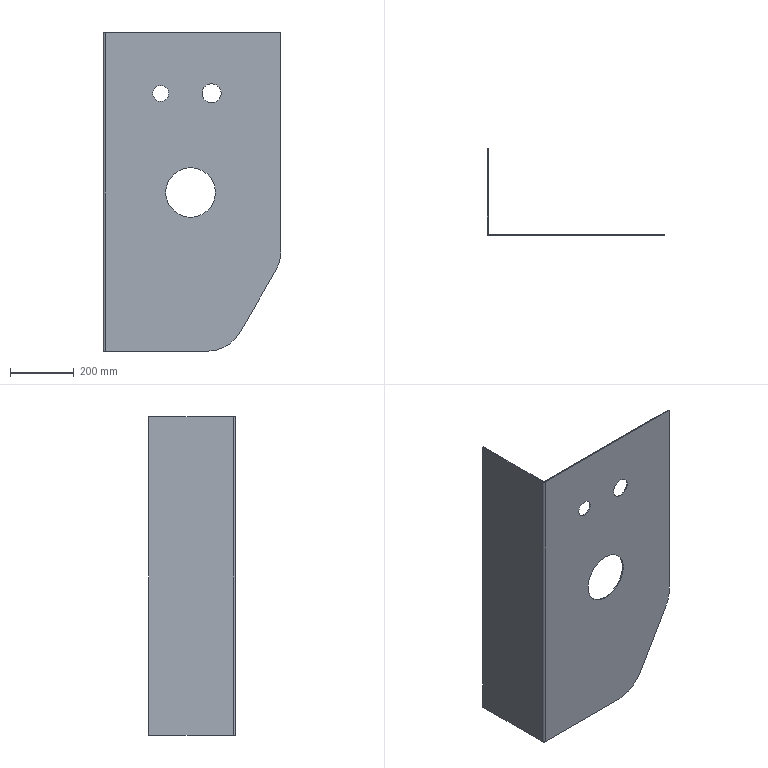Part | SolidWorks | features FlatPattern 1, ICE 1, SMBaseFlange 1, SheetMetal 1 | 1 solid | 24 faces | box 557 x 272 x 999 mm | volume 2327658 mm3 | plane 13 | cylinder 11 | commonest cylinder face diameters 6 x2 50 x2 60 x2 156 x2 234 x2 12 x1
STEP:
#1=CARTESIAN_POINT('',(274.,272.,420.));
#2=VERTEX_POINT('',#1);
#3=CARTESIAN_POINT('',(274.,272.,576.));
#4=VERTEX_POINT('',#3);
#5=CARTESIAN_POINT('',(274.,272.,498.));
#6=DIRECTION('',(0.,1.,0.));
#7=DIRECTION('',(0.,0.,1.));
#8=AXIS2_PLACEMENT_3D('',#5,#6,#7);
#9=CIRCLE('',#8,78.);
#10=EDGE_CURVE('',#2,#4,#9,.T.);
#11=ORIENTED_EDGE('',*,*,#10,.F.);
#12=CARTESIAN_POINT('',(274.,275.,420.));
#13=VERTEX_POINT('',#12);
#14=CARTESIAN_POINT('',(274.,275.,420.));
#15=DIRECTION('',(0.,1.,0.));
#16=VECTOR('',#15,1000.);
#17=LINE('',#14,#16);
#18=EDGE_CURVE('',#2,#13,#17,.T.);
#19=ORIENTED_EDGE('',*,*,#18,.T.);
#20=CARTESIAN_POINT('',(274.,275.,576.));
#21=VERTEX_POINT('',#20);
#22=CARTESIAN_POINT('',(274.,275.,498.));
#23=DIRECTION('',(0.,1.,0.));
#24=DIRECTION('',(0.,0.,1.));
#25=AXIS2_PLACEMENT_3D('',#22,#23,#24);
#26=CIRCLE('',#25,78.);
#27=EDGE_CURVE('',#13,#21,#26,.T.);
#28=ORIENTED_EDGE('',*,*,#27,.T.);
#29=CARTESIAN_POINT('',(274.,275.,576.));
#30=DIRECTION('',(0.,1.,0.));
#31=VECTOR('',#30,1000.);
#32=LINE('',#29,#31);
#33=EDGE_CURVE('',#4,#21,#32,.T.);
#34=ORIENTED_EDGE('',*,*,#33,.F.);
#35=EDGE_LOOP('',(#11,#19,#28,#34));
#36=FACE_OUTER_BOUND('',#35,.T.);
#37=CARTESIAN_POINT('',(274.,275.,498.));
#38=DIRECTION('',(0.,1.,0.));
#39=DIRECTION('',(0.,0.,1.));
#40=AXIS2_PLACEMENT_3D('',#37,#38,#39);
#41=CYLINDRICAL_SURFACE('',#40,78.);
#42=ADVANCED_FACE('',(#36),#41,.F.);
#43=CARTESIAN_POINT('',(340.,272.,779.));
#44=VERTEX_POINT('',#43);
#45=CARTESIAN_POINT('',(340.,272.,839.));
#46=VERTEX_POINT('',#45);
#47=CARTESIAN_POINT('',(340.,272.,809.));
#48=DIRECTION('',(0.,1.,0.));
#49=DIRECTION('',(0.,0.,1.));
#50=AXIS2_PLACEMENT_3D('',#47,#48,#49);
#51=CIRCLE('',#50,30.);
#52=EDGE_CURVE('',#44,#46,#51,.T.);
#53=ORIENTED_EDGE('',*,*,#52,.F.);
#54=CARTESIAN_POINT('',(340.,275.,779.));
#55=VERTEX_POINT('',#54);
#56=CARTESIAN_POINT('',(340.,275.,779.));
#57=DIRECTION('',(0.,1.,0.));
#58=VECTOR('',#57,1000.);
#59=LINE('',#56,#58);
#60=EDGE_CURVE('',#44,#55,#59,.T.);
#61=ORIENTED_EDGE('',*,*,#60,.T.);
#62=CARTESIAN_POINT('',(340.,275.,839.));
#63=VERTEX_POINT('',#62);
#64=CARTESIAN_POINT('',(340.,275.,809.));
#65=DIRECTION('',(0.,1.,0.));
#66=DIRECTION('',(0.,0.,1.));
#67=AXIS2_PLACEMENT_3D('',#64,#65,#66);
#68=CIRCLE('',#67,30.);
#69=EDGE_CURVE('',#55,#63,#68,.T.);
#70=ORIENTED_EDGE('',*,*,#69,.T.);
#71=CARTESIAN_POINT('',(340.,275.,839.));
#72=DIRECTION('',(0.,1.,0.));
#73=VECTOR('',#72,1000.);
#74=LINE('',#71,#73);
#75=EDGE_CURVE('',#46,#63,#74,.T.);
#76=ORIENTED_EDGE('',*,*,#75,.F.);
#77=EDGE_LOOP('',(#53,#61,#70,#76));
#78=FACE_OUTER_BOUND('',#77,.T.);
#79=CARTESIAN_POINT('',(340.,275.,809.));
#80=DIRECTION('',(0.,1.,0.));
#81=DIRECTION('',(0.,0.,1.));
#82=AXIS2_PLACEMENT_3D('',#79,#80,#81);
#83=CYLINDRICAL_SURFACE('',#82,30.);
#84=ADVANCED_FACE('',(#78),#83,.F.);
#85=CARTESIAN_POINT('',(180.,272.,784.));
#86=VERTEX_POINT('',#85);
#87=CARTESIAN_POINT('',(180.,272.,834.));
#88=VERTEX_POINT('',#87);
#89=CARTESIAN_POINT('',(180.,272.,809.));
#90=DIRECTION('',(0.,1.,0.));
#91=DIRECTION('',(0.,0.,1.));
#92=AXIS2_PLACEMENT_3D('',#89,#90,#91);
#93=CIRCLE('',#92,25.);
#94=EDGE_CURVE('',#86,#88,#93,.T.);
#95=ORIENTED_EDGE('',*,*,#94,.F.);
#96=CARTESIAN_POINT('',(180.,275.,784.));
#97=VERTEX_POINT('',#96);
#98=CARTESIAN_POINT('',(180.,275.,784.));
#99=DIRECTION('',(0.,1.,0.));
#100=VECTOR('',#99,1000.);
#101=LINE('',#98,#100);
#102=EDGE_CURVE('',#86,#97,#101,.T.);
#103=ORIENTED_EDGE('',*,*,#102,.T.);
#104=CARTESIAN_POINT('',(180.,275.,834.));
#105=VERTEX_POINT('',#104);
#106=CARTESIAN_POINT('',(180.,275.,809.));
#107=DIRECTION('',(0.,1.,0.));
#108=DIRECTION('',(0.,0.,1.));
#109=AXIS2_PLACEMENT_3D('',#106,#107,#108);
#110=CIRCLE('',#109,25.);
#111=EDGE_CURVE('',#97,#105,#110,.T.);
#112=ORIENTED_EDGE('',*,*,#111,.T.);
#113=CARTESIAN_POINT('',(180.,275.,834.));
#114=DIRECTION('',(0.,1.,0.));
#115=VECTOR('',#114,1000.);
#116=LINE('',#113,#115);
#117=EDGE_CURVE('',#88,#105,#116,.T.);
#118=ORIENTED_EDGE('',*,*,#117,.F.);
#119=EDGE_LOOP('',(#95,#103,#112,#118));
#120=FACE_OUTER_BOUND('',#119,.T.);
#121=CARTESIAN_POINT('',(180.,275.,809.));
#122=DIRECTION('',(0.,1.,0.));
#123=DIRECTION('',(0.,0.,1.));
#124=AXIS2_PLACEMENT_3D('',#121,#122,#123);
#125=CYLINDRICAL_SURFACE('',#124,25.);
#126=ADVANCED_FACE('',(#120),#125,.F.);
#127=CARTESIAN_POINT('',(274.,272.,498.));
#128=DIRECTION('',(0.,1.,0.));
#129=DIRECTION('',(0.,0.,1.));
#130=AXIS2_PLACEMENT_3D('',#127,#128,#129);
#131=CIRCLE('',#130,78.);
#132=EDGE_CURVE('',#4,#2,#131,.T.);
#133=ORIENTED_EDGE('',*,*,#132,.T.);
#134=ORIENTED_EDGE('',*,*,#10,.T.);
#135=EDGE_LOOP('',(#133,#134));
#136=FACE_BOUND('',#135,.T.);
#137=CARTESIAN_POINT('',(180.,272.,809.));
#138=DIRECTION('',(0.,1.,0.));
#139=DIRECTION('',(0.,0.,1.));
#140=AXIS2_PLACEMENT_3D('',#137,#138,#139);
#141=CIRCLE('',#140,25.);
#142=EDGE_CURVE('',#88,#86,#141,.T.);
#143=ORIENTED_EDGE('',*,*,#142,.T.);
#144=ORIENTED_EDGE('',*,*,#94,.T.);
#145=EDGE_LOOP('',(#143,#144));
#146=FACE_BOUND('',#145,.T.);
#147=CARTESIAN_POINT('',(340.,272.,809.));
#148=DIRECTION('',(0.,1.,0.));
#149=DIRECTION('',(0.,0.,1.));
#150=AXIS2_PLACEMENT_3D('',#147,#148,#149);
#151=CIRCLE('',#150,30.);
#152=EDGE_CURVE('',#46,#44,#151,.T.);
#153=ORIENTED_EDGE('',*,*,#152,.T.);
#154=ORIENTED_EDGE('',*,*,#52,.T.);
#155=EDGE_LOOP('',(#153,#154));
#156=FACE_BOUND('',#155,.T.);
#157=CARTESIAN_POINT('',(557.,272.,996.));
#158=VERTEX_POINT('',#157);
#159=CARTESIAN_POINT('',(554.,272.,999.));
#160=VERTEX_POINT('',#159);
#161=CARTESIAN_POINT('',(554.,272.,996.));
#162=DIRECTION('',(0.,-1.,0.));
#163=DIRECTION('',(0.,0.,1.));
#164=AXIS2_PLACEMENT_3D('',#161,#162,#163);
#165=CIRCLE('',#164,3.);
#166=EDGE_CURVE('',#158,#160,#165,.T.);
#167=ORIENTED_EDGE('',*,*,#166,.T.);
#168=CARTESIAN_POINT('',(6.,272.,999.));
#169=VERTEX_POINT('',#168);
#170=CARTESIAN_POINT('',(0.,272.,999.));
#171=DIRECTION('',(1.,0.,0.));
#172=VECTOR('',#171,1000.);
#173=LINE('',#170,#172);
#174=EDGE_CURVE('',#169,#160,#173,.T.);
#175=ORIENTED_EDGE('',*,*,#174,.F.);
#176=CARTESIAN_POINT('',(6.,272.,0.));
#177=VERTEX_POINT('',#176);
#178=CARTESIAN_POINT('',(6.,272.,999.));
#179=DIRECTION('',(0.,0.,-1.));
#180=VECTOR('',#179,1000.);
#181=LINE('',#178,#180);
#182=EDGE_CURVE('',#169,#177,#181,.T.);
#183=ORIENTED_EDGE('',*,*,#182,.T.);
#184=CARTESIAN_POINT('',(327.792,272.,0.));
#185=VERTEX_POINT('',#184);
#186=CARTESIAN_POINT('',(0.,272.,0.));
#187=DIRECTION('',(1.,0.,0.));
#188=VECTOR('',#187,1000.);
#189=LINE('',#186,#188);
#190=EDGE_CURVE('',#177,#185,#189,.T.);
#191=ORIENTED_EDGE('',*,*,#190,.T.);
#192=CARTESIAN_POINT('',(429.117,272.,58.5));
#193=VERTEX_POINT('',#192);
#194=CARTESIAN_POINT('',(327.792,272.,117.));
#195=DIRECTION('',(0.,-1.,0.));
#196=DIRECTION('',(0.,0.,1.));
#197=AXIS2_PLACEMENT_3D('',#194,#195,#196);
#198=CIRCLE('',#197,117.);
#199=EDGE_CURVE('',#185,#193,#198,.T.);
#200=ORIENTED_EDGE('',*,*,#199,.T.);
#201=CARTESIAN_POINT('',(541.325,272.,252.85));
#202=VERTEX_POINT('',#201);
#203=CARTESIAN_POINT('',(729.086,272.,578.062));
#204=DIRECTION('',(0.5,0.,0.866));
#205=VECTOR('',#204,1000.);
#206=LINE('',#203,#205);
#207=EDGE_CURVE('',#193,#202,#206,.T.);
#208=ORIENTED_EDGE('',*,*,#207,.T.);
#209=CARTESIAN_POINT('',(557.,272.,311.35));
#210=VERTEX_POINT('',#209);
#211=CARTESIAN_POINT('',(440.,272.,311.35));
#212=DIRECTION('',(0.,-1.,0.));
#213=DIRECTION('',(0.,0.,1.));
#214=AXIS2_PLACEMENT_3D('',#211,#212,#213);
#215=CIRCLE('',#214,117.);
#216=EDGE_CURVE('',#202,#210,#215,.T.);
#217=ORIENTED_EDGE('',*,*,#216,.T.);
#218=CARTESIAN_POINT('',(557.,272.,999.));
#219=DIRECTION('',(0.,0.,-1.));
#220=VECTOR('',#219,1000.);
#221=LINE('',#218,#220);
#222=EDGE_CURVE('',#158,#210,#221,.T.);
#223=ORIENTED_EDGE('',*,*,#222,.F.);
#224=EDGE_LOOP('',(#167,#175,#183,#191,#200,#208,#217,#223));
#225=FACE_OUTER_BOUND('',#224,.T.);
#226=CARTESIAN_POINT('',(0.,272.,999.));
#227=DIRECTION('',(0.,1.,0.));
#228=DIRECTION('',(0.,0.,1.));
#229=AXIS2_PLACEMENT_3D('',#226,#227,#228);
#230=PLANE('',#229);
#231=ADVANCED_FACE('',(#136,#146,#156,#225),#230,.F.);
#232=CARTESIAN_POINT('',(274.,275.,498.));
#233=DIRECTION('',(0.,1.,0.));
#234=DIRECTION('',(0.,0.,1.));
#235=AXIS2_PLACEMENT_3D('',#232,#233,#234);
#236=CIRCLE('',#235,78.);
#237=EDGE_CURVE('',#21,#13,#236,.T.);
#238=ORIENTED_EDGE('',*,*,#237,.F.);
#239=ORIENTED_EDGE('',*,*,#27,.F.);
#240=EDGE_LOOP('',(#238,#239));
#241=FACE_BOUND('',#240,.T.);
#242=CARTESIAN_POINT('',(180.,275.,809.));
#243=DIRECTION('',(0.,1.,0.));
#244=DIRECTION('',(0.,0.,1.));
#245=AXIS2_PLACEMENT_3D('',#242,#243,#244);
#246=CIRCLE('',#245,25.);
#247=EDGE_CURVE('',#105,#97,#246,.T.);
#248=ORIENTED_EDGE('',*,*,#247,.F.);
#249=ORIENTED_EDGE('',*,*,#111,.F.);
#250=EDGE_LOOP('',(#248,#249));
#251=FACE_BOUND('',#250,.T.);
#252=CARTESIAN_POINT('',(340.,275.,809.));
#253=DIRECTION('',(0.,1.,0.));
#254=DIRECTION('',(0.,0.,1.));
#255=AXIS2_PLACEMENT_3D('',#252,#253,#254);
#256=CIRCLE('',#255,30.);
#257=EDGE_CURVE('',#63,#55,#256,.T.);
#258=ORIENTED_EDGE('',*,*,#257,.F.);
#259=ORIENTED_EDGE('',*,*,#69,.F.);
#260=EDGE_LOOP('',(#258,#259));
#261=FACE_BOUND('',#260,.T.);
#262=CARTESIAN_POINT('',(6.,275.,999.));
#263=VERTEX_POINT('',#262);
#264=CARTESIAN_POINT('',(554.,275.,999.));
#265=VERTEX_POINT('',#264);
#266=CARTESIAN_POINT('',(0.,275.,999.));
#267=DIRECTION('',(1.,0.,0.));
#268=VECTOR('',#267,1000.);
#269=LINE('',#266,#268);
#270=EDGE_CURVE('',#263,#265,#269,.T.);
#271=ORIENTED_EDGE('',*,*,#270,.T.);
#272=CARTESIAN_POINT('',(557.,275.,996.));
#273=VERTEX_POINT('',#272);
#274=CARTESIAN_POINT('',(554.,275.,996.));
#275=DIRECTION('',(0.,-1.,0.));
#276=DIRECTION('',(0.,0.,1.));
#277=AXIS2_PLACEMENT_3D('',#274,#275,#276);
#278=CIRCLE('',#277,3.);
#279=EDGE_CURVE('',#273,#265,#278,.T.);
#280=ORIENTED_EDGE('',*,*,#279,.F.);
#281=CARTESIAN_POINT('',(557.,275.,311.35));
#282=VERTEX_POINT('',#281);
#283=CARTESIAN_POINT('',(557.,275.,999.));
#284=DIRECTION('',(0.,0.,-1.));
#285=VECTOR('',#284,1000.);
#286=LINE('',#283,#285);
#287=EDGE_CURVE('',#273,#282,#286,.T.);
#288=ORIENTED_EDGE('',*,*,#287,.T.);
#289=CARTESIAN_POINT('',(541.325,275.,252.85));
#290=VERTEX_POINT('',#289);
#291=CARTESIAN_POINT('',(440.,275.,311.35));
#292=DIRECTION('',(0.,-1.,0.));
#293=DIRECTION('',(0.,0.,1.));
#294=AXIS2_PLACEMENT_3D('',#291,#292,#293);
#295=CIRCLE('',#294,117.);
#296=EDGE_CURVE('',#290,#282,#295,.T.);
#297=ORIENTED_EDGE('',*,*,#296,.F.);
#298=CARTESIAN_POINT('',(429.117,275.,58.5));
#299=VERTEX_POINT('',#298);
#300=CARTESIAN_POINT('',(729.086,275.,578.062));
#301=DIRECTION('',(0.5,0.,0.866));
#302=VECTOR('',#301,1000.);
#303=LINE('',#300,#302);
#304=EDGE_CURVE('',#299,#290,#303,.T.);
#305=ORIENTED_EDGE('',*,*,#304,.F.);
#306=CARTESIAN_POINT('',(327.792,275.,0.));
#307=VERTEX_POINT('',#306);
#308=CARTESIAN_POINT('',(327.792,275.,117.));
#309=DIRECTION('',(0.,-1.,0.));
#310=DIRECTION('',(0.,0.,1.));
#311=AXIS2_PLACEMENT_3D('',#308,#309,#310);
#312=CIRCLE('',#311,117.);
#313=EDGE_CURVE('',#307,#299,#312,.T.);
#314=ORIENTED_EDGE('',*,*,#313,.F.);
#315=CARTESIAN_POINT('',(6.,275.,0.));
#316=VERTEX_POINT('',#315);
#317=CARTESIAN_POINT('',(0.,275.,0.));
#318=DIRECTION('',(1.,0.,0.));
#319=VECTOR('',#318,1000.);
#320=LINE('',#317,#319);
#321=EDGE_CURVE('',#316,#307,#320,.T.);
#322=ORIENTED_EDGE('',*,*,#321,.F.);
#323=CARTESIAN_POINT('',(6.,275.,999.));
#324=DIRECTION('',(0.,0.,-1.));
#325=VECTOR('',#324,1000.);
#326=LINE('',#323,#325);
#327=EDGE_CURVE('',#263,#316,#326,.T.);
#328=ORIENTED_EDGE('',*,*,#327,.F.);
#329=EDGE_LOOP('',(#271,#280,#288,#297,#305,#314,#322,#328));
#330=FACE_OUTER_BOUND('',#329,.T.);
#331=CARTESIAN_POINT('',(0.,275.,999.));
#332=DIRECTION('',(0.,1.,0.));
#333=DIRECTION('',(0.,0.,1.));
#334=AXIS2_PLACEMENT_3D('',#331,#332,#333);
#335=PLANE('',#334);
#336=ADVANCED_FACE('',(#241,#251,#261,#330),#335,.T.);
#337=ORIENTED_EDGE('',*,*,#174,.T.);
#338=CARTESIAN_POINT('',(554.,275.,999.));
#339=DIRECTION('',(0.,-1.,0.));
#340=VECTOR('',#339,1000.);
#341=LINE('',#338,#340);
#342=EDGE_CURVE('',#265,#160,#341,.T.);
#343=ORIENTED_EDGE('',*,*,#342,.F.);
#344=ORIENTED_EDGE('',*,*,#270,.F.);
#345=CARTESIAN_POINT('',(6.,275.,999.));
#346=DIRECTION('',(0.,-1.,0.));
#347=VECTOR('',#346,1000.);
#348=LINE('',#345,#347);
#349=EDGE_CURVE('',#263,#169,#348,.T.);
#350=ORIENTED_EDGE('',*,*,#349,.T.);
#351=EDGE_LOOP('',(#337,#343,#344,#350));
#352=FACE_OUTER_BOUND('',#351,.T.);
#353=CARTESIAN_POINT('',(6.,278.,999.));
#354=DIRECTION('',(0.,0.,1.));
#355=DIRECTION('',(1.,0.,0.));
#356=AXIS2_PLACEMENT_3D('',#353,#354,#355);
#357=PLANE('',#356);
#358=ADVANCED_FACE('',(#352),#357,.T.);
#359=CARTESIAN_POINT('',(557.,275.,996.));
#360=DIRECTION('',(0.,-1.,0.));
#361=VECTOR('',#360,1000.);
#362=LINE('',#359,#361);
#363=EDGE_CURVE('',#273,#158,#362,.T.);
#364=ORIENTED_EDGE('',*,*,#363,.T.);
#365=ORIENTED_EDGE('',*,*,#222,.T.);
#366=CARTESIAN_POINT('',(557.,275.,311.35));
#367=DIRECTION('',(0.,-1.,0.));
#368=VECTOR('',#367,1000.);
#369=LINE('',#366,#368);
#370=EDGE_CURVE('',#282,#210,#369,.T.);
#371=ORIENTED_EDGE('',*,*,#370,.F.);
#372=ORIENTED_EDGE('',*,*,#287,.F.);
#373=EDGE_LOOP('',(#364,#365,#371,#372));
#374=FACE_OUTER_BOUND('',#373,.T.);
#375=CARTESIAN_POINT('',(557.,275.,999.));
#376=DIRECTION('',(1.,0.,0.));
#377=DIRECTION('',(0.,0.,-1.));
#378=AXIS2_PLACEMENT_3D('',#375,#376,#377);
#379=PLANE('',#378);
#380=ADVANCED_FACE('',(#374),#379,.T.);
#381=CARTESIAN_POINT('',(0.,278.,999.));
#382=VERTEX_POINT('',#381);
#383=CARTESIAN_POINT('',(3.,278.,999.));
#384=VERTEX_POINT('',#383);
#385=CARTESIAN_POINT('',(0.,278.,999.));
#386=DIRECTION('',(1.,0.,0.));
#387=VECTOR('',#386,1000.);
#388=LINE('',#385,#387);
#389=EDGE_CURVE('',#382,#384,#388,.T.);
#390=ORIENTED_EDGE('',*,*,#389,.F.);
#391=CARTESIAN_POINT('',(6.,278.,999.));
#392=DIRECTION('',(0.,0.,1.));
#393=DIRECTION('',(1.,0.,0.));
#394=AXIS2_PLACEMENT_3D('',#391,#392,#393);
#395=CIRCLE('',#394,6.);
#396=EDGE_CURVE('',#382,#169,#395,.T.);
#397=ORIENTED_EDGE('',*,*,#396,.T.);
#398=ORIENTED_EDGE('',*,*,#349,.F.);
#399=CARTESIAN_POINT('',(6.,278.,999.));
#400=DIRECTION('',(0.,0.,1.));
#401=DIRECTION('',(1.,0.,0.));
#402=AXIS2_PLACEMENT_3D('',#399,#400,#401);
#403=CIRCLE('',#402,3.);
#404=EDGE_CURVE('',#384,#263,#403,.T.);
#405=ORIENTED_EDGE('',*,*,#404,.F.);
#406=EDGE_LOOP('',(#390,#397,#398,#405));
#407=FACE_OUTER_BOUND('',#406,.T.);
#408=CARTESIAN_POINT('',(0.,278.,999.));
#409=DIRECTION('',(0.,0.,1.));
#410=DIRECTION('',(1.,0.,0.));
#411=AXIS2_PLACEMENT_3D('',#408,#409,#410);
#412=PLANE('',#411);
#413=ADVANCED_FACE('',(#407),#412,.T.);
#414=CARTESIAN_POINT('',(0.,544.,999.));
#415=VERTEX_POINT('',#414);
#416=CARTESIAN_POINT('',(0.,272.,999.));
#417=DIRECTION('',(0.,-1.,0.));
#418=VECTOR('',#417,1000.);
#419=LINE('',#416,#418);
#420=EDGE_CURVE('',#415,#382,#419,.T.);
#421=ORIENTED_EDGE('',*,*,#420,.T.);
#422=ORIENTED_EDGE('',*,*,#389,.T.);
#423=CARTESIAN_POINT('',(3.,544.,999.));
#424=VERTEX_POINT('',#423);
#425=CARTESIAN_POINT('',(3.,272.,999.));
#426=DIRECTION('',(0.,-1.,0.));
#427=VECTOR('',#426,1000.);
#428=LINE('',#425,#427);
#429=EDGE_CURVE('',#424,#384,#428,.T.);
#430=ORIENTED_EDGE('',*,*,#429,.F.);
#431=CARTESIAN_POINT('',(0.,544.,999.));
#432=DIRECTION('',(1.,0.,0.));
#433=VECTOR('',#432,1000.);
#434=LINE('',#431,#433);
#435=EDGE_CURVE('',#415,#424,#434,.T.);
#436=ORIENTED_EDGE('',*,*,#435,.F.);
#437=EDGE_LOOP('',(#421,#422,#430,#436));
#438=FACE_OUTER_BOUND('',#437,.T.);
#439=CARTESIAN_POINT('',(6.,275.,999.));
#440=DIRECTION('',(0.,0.,1.));
#441=DIRECTION('',(1.,0.,0.));
#442=AXIS2_PLACEMENT_3D('',#439,#440,#441);
#443=PLANE('',#442);
#444=ADVANCED_FACE('',(#438),#443,.T.);
#445=CARTESIAN_POINT('',(6.,272.,0.));
#446=DIRECTION('',(0.,1.,0.));
#447=VECTOR('',#446,1000.);
#448=LINE('',#445,#447);
#449=EDGE_CURVE('',#177,#316,#448,.T.);
#450=ORIENTED_EDGE('',*,*,#449,.F.);
#451=CARTESIAN_POINT('',(0.,278.,0.));
#452=VERTEX_POINT('',#451);
#453=CARTESIAN_POINT('',(6.,278.,0.));
#454=DIRECTION('',(0.,0.,1.));
#455=DIRECTION('',(1.,0.,0.));
#456=AXIS2_PLACEMENT_3D('',#453,#454,#455);
#457=CIRCLE('',#456,6.);
#458=EDGE_CURVE('',#452,#177,#457,.T.);
#459=ORIENTED_EDGE('',*,*,#458,.F.);
#460=CARTESIAN_POINT('',(3.,278.,0.));
#461=VERTEX_POINT('',#460);
#462=CARTESIAN_POINT('',(3.,278.,0.));
#463=DIRECTION('',(-1.,0.,0.));
#464=VECTOR('',#463,1000.);
#465=LINE('',#462,#464);
#466=EDGE_CURVE('',#461,#452,#465,.T.);
#467=ORIENTED_EDGE('',*,*,#466,.F.);
#468=CARTESIAN_POINT('',(6.,278.,0.));
#469=DIRECTION('',(0.,0.,1.));
#470=DIRECTION('',(1.,0.,0.));
#471=AXIS2_PLACEMENT_3D('',#468,#469,#470);
#472=CIRCLE('',#471,3.);
#473=EDGE_CURVE('',#461,#316,#472,.T.);
#474=ORIENTED_EDGE('',*,*,#473,.T.);
#475=EDGE_LOOP('',(#450,#459,#467,#474));
#476=FACE_OUTER_BOUND('',#475,.T.);
#477=CARTESIAN_POINT('',(6.,272.,0.));
#478=DIRECTION('',(0.,0.,-1.));
#479=DIRECTION('',(-1.,0.,0.));
#480=AXIS2_PLACEMENT_3D('',#477,#478,#479);
#481=PLANE('',#480);
#482=ADVANCED_FACE('',(#476),#481,.T.);
#483=CARTESIAN_POINT('',(327.792,275.,0.));
#484=DIRECTION('',(0.,-1.,0.));
#485=VECTOR('',#484,1000.);
#486=LINE('',#483,#485);
#487=EDGE_CURVE('',#307,#185,#486,.T.);
#488=ORIENTED_EDGE('',*,*,#487,.T.);
#489=ORIENTED_EDGE('',*,*,#190,.F.);
#490=ORIENTED_EDGE('',*,*,#449,.T.);
#491=ORIENTED_EDGE('',*,*,#321,.T.);
#492=EDGE_LOOP('',(#488,#489,#490,#491));
#493=FACE_OUTER_BOUND('',#492,.T.);
#494=CARTESIAN_POINT('',(3.,278.,0.));
#495=DIRECTION('',(0.,0.,-1.));
#496=DIRECTION('',(-1.,0.,0.));
#497=AXIS2_PLACEMENT_3D('',#494,#495,#496);
#498=PLANE('',#497);
#499=ADVANCED_FACE('',(#493),#498,.T.);
#500=ORIENTED_EDGE('',*,*,#473,.F.);
#501=CARTESIAN_POINT('',(3.,278.,999.));
#502=DIRECTION('',(0.,0.,-1.));
#503=VECTOR('',#502,1000.);
#504=LINE('',#501,#503);
#505=EDGE_CURVE('',#384,#461,#504,.T.);
#506=ORIENTED_EDGE('',*,*,#505,.F.);
#507=ORIENTED_EDGE('',*,*,#404,.T.);
#508=ORIENTED_EDGE('',*,*,#327,.T.);
#509=EDGE_LOOP('',(#500,#506,#507,#508));
#510=FACE_OUTER_BOUND('',#509,.T.);
#511=CARTESIAN_POINT('',(6.,278.,999.));
#512=DIRECTION('',(0.,0.,-1.));
#513=DIRECTION('',(-1.,0.,0.));
#514=AXIS2_PLACEMENT_3D('',#511,#512,#513);
#515=CYLINDRICAL_SURFACE('',#514,3.);
#516=ADVANCED_FACE('',(#510),#515,.F.);
#517=CARTESIAN_POINT('',(3.,544.,0.));
#518=VERTEX_POINT('',#517);
#519=CARTESIAN_POINT('',(3.,272.,0.));
#520=DIRECTION('',(0.,-1.,0.));
#521=VECTOR('',#520,1000.);
#522=LINE('',#519,#521);
#523=EDGE_CURVE('',#518,#461,#522,.T.);
#524=ORIENTED_EDGE('',*,*,#523,.F.);
#525=CARTESIAN_POINT('',(3.,544.,999.));
#526=DIRECTION('',(0.,0.,-1.));
#527=VECTOR('',#526,1000.);
#528=LINE('',#525,#527);
#529=EDGE_CURVE('',#424,#518,#528,.T.);
#530=ORIENTED_EDGE('',*,*,#529,.F.);
#531=ORIENTED_EDGE('',*,*,#429,.T.);
#532=ORIENTED_EDGE('',*,*,#505,.T.);
#533=EDGE_LOOP('',(#524,#530,#531,#532));
#534=FACE_OUTER_BOUND('',#533,.T.);
#535=CARTESIAN_POINT('',(3.,272.,999.));
#536=DIRECTION('',(1.,0.,0.));
#537=DIRECTION('',(0.,0.,-1.));
#538=AXIS2_PLACEMENT_3D('',#535,#536,#537);
#539=PLANE('',#538);
#540=ADVANCED_FACE('',(#534),#539,.T.);
#541=CARTESIAN_POINT('',(0.,544.,0.));
#542=VERTEX_POINT('',#541);
#543=CARTESIAN_POINT('',(0.,544.,0.));
#544=DIRECTION('',(1.,0.,0.));
#545=VECTOR('',#544,1000.);
#546=LINE('',#543,#545);
#547=EDGE_CURVE('',#542,#518,#546,.T.);
#548=ORIENTED_EDGE('',*,*,#547,.F.);
#549=CARTESIAN_POINT('',(0.,544.,999.));
#550=DIRECTION('',(0.,0.,-1.));
#551=VECTOR('',#550,1000.);
#552=LINE('',#549,#551);
#553=EDGE_CURVE('',#415,#542,#552,.T.);
#554=ORIENTED_EDGE('',*,*,#553,.F.);
#555=ORIENTED_EDGE('',*,*,#435,.T.);
#556=ORIENTED_EDGE('',*,*,#529,.T.);
#557=EDGE_LOOP('',(#548,#554,#555,#556));
#558=FACE_OUTER_BOUND('',#557,.T.);
#559=CARTESIAN_POINT('',(0.,544.,999.));
#560=DIRECTION('',(0.,1.,0.));
#561=DIRECTION('',(0.,0.,1.));
#562=AXIS2_PLACEMENT_3D('',#559,#560,#561);
#563=PLANE('',#562);
#564=ADVANCED_FACE('',(#558),#563,.T.);
#565=CARTESIAN_POINT('',(0.,272.,0.));
#566=DIRECTION('',(0.,-1.,0.));
#567=VECTOR('',#566,1000.);
#568=LINE('',#565,#567);
#569=EDGE_CURVE('',#542,#452,#568,.T.);
#570=ORIENTED_EDGE('',*,*,#569,.T.);
#571=CARTESIAN_POINT('',(0.,278.,999.));
#572=DIRECTION('',(0.,0.,-1.));
#573=VECTOR('',#572,1000.);
#574=LINE('',#571,#573);
#575=EDGE_CURVE('',#382,#452,#574,.T.);
#576=ORIENTED_EDGE('',*,*,#575,.F.);
#577=ORIENTED_EDGE('',*,*,#420,.F.);
#578=ORIENTED_EDGE('',*,*,#553,.T.);
#579=EDGE_LOOP('',(#570,#576,#577,#578));
#580=FACE_OUTER_BOUND('',#579,.T.);
#581=CARTESIAN_POINT('',(0.,272.,999.));
#582=DIRECTION('',(1.,0.,0.));
#583=DIRECTION('',(0.,0.,-1.));
#584=AXIS2_PLACEMENT_3D('',#581,#582,#583);
#585=PLANE('',#584);
#586=ADVANCED_FACE('',(#580),#585,.F.);
#587=ORIENTED_EDGE('',*,*,#458,.T.);
#588=ORIENTED_EDGE('',*,*,#182,.F.);
#589=ORIENTED_EDGE('',*,*,#396,.F.);
#590=ORIENTED_EDGE('',*,*,#575,.T.);
#591=EDGE_LOOP('',(#587,#588,#589,#590));
#592=FACE_OUTER_BOUND('',#591,.T.);
#593=CARTESIAN_POINT('',(6.,278.,999.));
#594=DIRECTION('',(0.,0.,-1.));
#595=DIRECTION('',(-1.,0.,0.));
#596=AXIS2_PLACEMENT_3D('',#593,#594,#595);
#597=CYLINDRICAL_SURFACE('',#596,6.);
#598=ADVANCED_FACE('',(#592),#597,.T.);
#599=ORIENTED_EDGE('',*,*,#523,.T.);
#600=ORIENTED_EDGE('',*,*,#466,.T.);
#601=ORIENTED_EDGE('',*,*,#569,.F.);
#602=ORIENTED_EDGE('',*,*,#547,.T.);
#603=EDGE_LOOP('',(#599,#600,#601,#602));
#604=FACE_OUTER_BOUND('',#603,.T.);
#605=CARTESIAN_POINT('',(6.,278.,0.));
#606=DIRECTION('',(0.,0.,1.));
#607=DIRECTION('',(1.,0.,0.));
#608=AXIS2_PLACEMENT_3D('',#605,#606,#607);
#609=PLANE('',#608);
#610=ADVANCED_FACE('',(#604),#609,.F.);
#611=CARTESIAN_POINT('',(429.117,275.,58.5));
#612=DIRECTION('',(0.,-1.,0.));
#613=VECTOR('',#612,1000.);
#614=LINE('',#611,#613);
#615=EDGE_CURVE('',#299,#193,#614,.T.);
#616=ORIENTED_EDGE('',*,*,#615,.F.);
#617=ORIENTED_EDGE('',*,*,#304,.T.);
#618=CARTESIAN_POINT('',(541.325,275.,252.85));
#619=DIRECTION('',(0.,-1.,0.));
#620=VECTOR('',#619,1000.);
#621=LINE('',#618,#620);
#622=EDGE_CURVE('',#290,#202,#621,.T.);
#623=ORIENTED_EDGE('',*,*,#622,.T.);
#624=ORIENTED_EDGE('',*,*,#207,.F.);
#625=EDGE_LOOP('',(#616,#617,#623,#624));
#626=FACE_OUTER_BOUND('',#625,.T.);
#627=CARTESIAN_POINT('',(729.086,275.,578.062));
#628=DIRECTION('',(-0.866,0.,0.5));
#629=DIRECTION('',(0.5,0.,0.866));
#630=AXIS2_PLACEMENT_3D('',#627,#628,#629);
#631=PLANE('',#630);
#632=ADVANCED_FACE('',(#626),#631,.F.);
#633=ORIENTED_EDGE('',*,*,#622,.F.);
#634=ORIENTED_EDGE('',*,*,#296,.T.);
#635=ORIENTED_EDGE('',*,*,#370,.T.);
#636=ORIENTED_EDGE('',*,*,#216,.F.);
#637=EDGE_LOOP('',(#633,#634,#635,#636));
#638=FACE_OUTER_BOUND('',#637,.T.);
#639=CARTESIAN_POINT('',(440.,275.,311.35));
#640=DIRECTION('',(0.,1.,0.));
#641=DIRECTION('',(0.,0.,1.));
#642=AXIS2_PLACEMENT_3D('',#639,#640,#641);
#643=CYLINDRICAL_SURFACE('',#642,117.);
#644=ADVANCED_FACE('',(#638),#643,.T.);
#645=ORIENTED_EDGE('',*,*,#313,.T.);
#646=ORIENTED_EDGE('',*,*,#615,.T.);
#647=ORIENTED_EDGE('',*,*,#199,.F.);
#648=ORIENTED_EDGE('',*,*,#487,.F.);
#649=EDGE_LOOP('',(#645,#646,#647,#648));
#650=FACE_OUTER_BOUND('',#649,.T.);
#651=CARTESIAN_POINT('',(327.792,275.,117.));
#652=DIRECTION('',(0.,1.,0.));
#653=DIRECTION('',(0.,0.,1.));
#654=AXIS2_PLACEMENT_3D('',#651,#652,#653);
#655=CYLINDRICAL_SURFACE('',#654,117.);
#656=ADVANCED_FACE('',(#650),#655,.T.);
#657=ORIENTED_EDGE('',*,*,#102,.F.);
#658=ORIENTED_EDGE('',*,*,#142,.F.);
#659=ORIENTED_EDGE('',*,*,#117,.T.);
#660=ORIENTED_EDGE('',*,*,#247,.T.);
#661=EDGE_LOOP('',(#657,#658,#659,#660));
#662=FACE_OUTER_BOUND('',#661,.T.);
#663=CARTESIAN_POINT('',(180.,275.,809.));
#664=DIRECTION('',(0.,1.,0.));
#665=DIRECTION('',(0.,0.,1.));
#666=AXIS2_PLACEMENT_3D('',#663,#664,#665);
#667=CYLINDRICAL_SURFACE('',#666,25.);
#668=ADVANCED_FACE('',(#662),#667,.F.);
#669=ORIENTED_EDGE('',*,*,#60,.F.);
#670=ORIENTED_EDGE('',*,*,#152,.F.);
#671=ORIENTED_EDGE('',*,*,#75,.T.);
#672=ORIENTED_EDGE('',*,*,#257,.T.);
#673=EDGE_LOOP('',(#669,#670,#671,#672));
#674=FACE_OUTER_BOUND('',#673,.T.);
#675=CARTESIAN_POINT('',(340.,275.,809.));
#676=DIRECTION('',(0.,1.,0.));
#677=DIRECTION('',(0.,0.,1.));
#678=AXIS2_PLACEMENT_3D('',#675,#676,#677);
#679=CYLINDRICAL_SURFACE('',#678,30.);
#680=ADVANCED_FACE('',(#674),#679,.F.);
#681=ORIENTED_EDGE('',*,*,#18,.F.);
#682=ORIENTED_EDGE('',*,*,#132,.F.);
#683=ORIENTED_EDGE('',*,*,#33,.T.);
#684=ORIENTED_EDGE('',*,*,#237,.T.);
#685=EDGE_LOOP('',(#681,#682,#683,#684));
#686=FACE_OUTER_BOUND('',#685,.T.);
#687=CARTESIAN_POINT('',(274.,275.,498.));
#688=DIRECTION('',(0.,1.,0.));
#689=DIRECTION('',(0.,0.,1.));
#690=AXIS2_PLACEMENT_3D('',#687,#688,#689);
#691=CYLINDRICAL_SURFACE('',#690,78.);
#692=ADVANCED_FACE('',(#686),#691,.F.);
#693=ORIENTED_EDGE('',*,*,#279,.T.);
#694=ORIENTED_EDGE('',*,*,#342,.T.);
#695=ORIENTED_EDGE('',*,*,#166,.F.);
#696=ORIENTED_EDGE('',*,*,#363,.F.);
#697=EDGE_LOOP('',(#693,#694,#695,#696));
#698=FACE_OUTER_BOUND('',#697,.T.);
#699=CARTESIAN_POINT('',(554.,275.,996.));
#700=DIRECTION('',(0.,1.,0.));
#701=DIRECTION('',(0.,0.,1.));
#702=AXIS2_PLACEMENT_3D('',#699,#700,#701);
#703=CYLINDRICAL_SURFACE('',#702,3.);
#704=ADVANCED_FACE('',(#698),#703,.T.);
#705=CLOSED_SHELL('',(#42,#84,#126,#231,#336,#358,#380,#413,#444,#482,#499,#516,#540,#564,#586,#598,#610,#632,#644,#656,#668,#680,#692,#704));
#706=MANIFOLD_SOLID_BREP('',#705);
#707=CARTESIAN_POINT('',(0.,0.,0.));
#708=DIRECTION('',(0.,0.,1.));
#709=DIRECTION('',(1.,0.,0.));
#710=AXIS2_PLACEMENT_3D('',#707,#708,#709);
#711=(LENGTH_UNIT()NAMED_UNIT(*)SI_UNIT(.MILLI.,.METRE.));
#712=UNCERTAINTY_MEASURE_WITH_UNIT(LENGTH_MEASURE(0.00001),#711,'','');
#713=(NAMED_UNIT(*)PLANE_ANGLE_UNIT()SI_UNIT($,.RADIAN.));
#714=(NAMED_UNIT(*)SI_UNIT($,.STERADIAN.)SOLID_ANGLE_UNIT());
#715=(GEOMETRIC_REPRESENTATION_CONTEXT(3)GLOBAL_UNCERTAINTY_ASSIGNED_CONTEXT((#712))GLOBAL_UNIT_ASSIGNED_CONTEXT((#711,#713,#714))REPRESENTATION_CONTEXT('',''));
#716=ADVANCED_BREP_SHAPE_REPRESENTATION('',(#706,#710),#715);